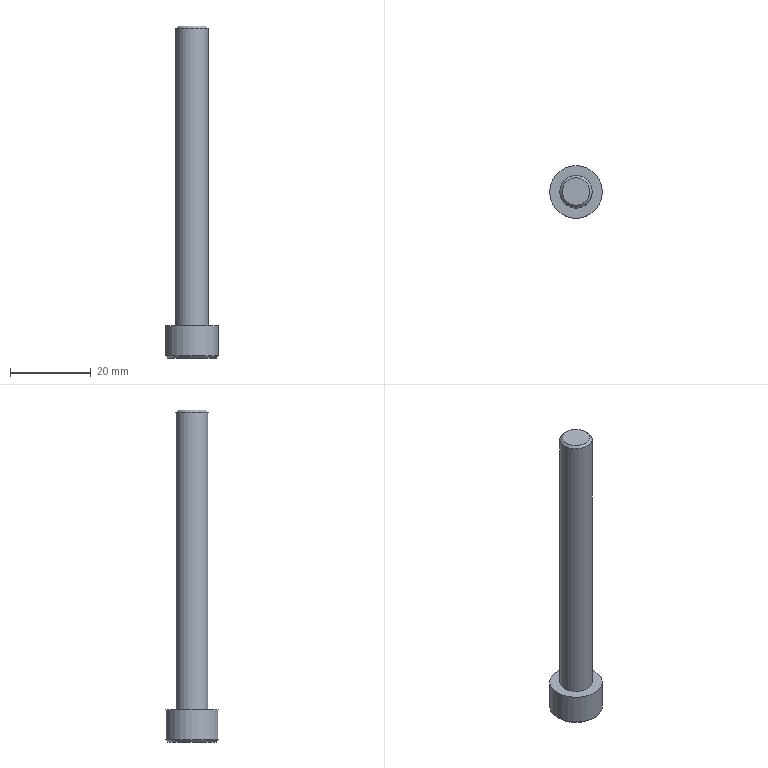Part | STEP file | gslz 2016.10.28-6_id182_x_t | 1 solid | 14 faces | box 13 x 13 x 82 mm | volume 4616 mm3 | plane 10 | cylinder 2 | cone 2 | commonest cylinder face diameters 8 x1 13 x1
STEP:
#1=CARTESIAN_POINT('',(-246.,150.,62.992));
#2=VERTEX_POINT('',#1);
#3=CARTESIAN_POINT('',(-240.,150.,62.992));
#4=DIRECTION('',(0.,0.,-1.));
#5=DIRECTION('',(-1.,0.,0.));
#6=AXIS2_PLACEMENT_3D('',#3,#4,#5);
#7=CIRCLE('',#6,6.);
#8=EDGE_CURVE('',#2,#2,#7,.T.);
#9=ORIENTED_EDGE('',*,*,#8,.T.);
#10=EDGE_LOOP('',(#9));
#11=FACE_BOUND('',#10,.T.);
#12=CARTESIAN_POINT('',(-237.,151.732,62.992));
#13=VERTEX_POINT('',#12);
#14=CARTESIAN_POINT('',(-237.,148.268,62.992));
#15=VERTEX_POINT('',#14);
#16=CARTESIAN_POINT('',(-237.,151.732,62.992));
#17=DIRECTION('',(0.,-1.,0.));
#18=VECTOR('',#17,1.);
#19=LINE('',#16,#18);
#20=EDGE_CURVE('',#13,#15,#19,.T.);
#21=ORIENTED_EDGE('',*,*,#20,.F.);
#22=CARTESIAN_POINT('',(-240.,153.464,62.992));
#23=VERTEX_POINT('',#22);
#24=CARTESIAN_POINT('',(-240.,153.464,62.992));
#25=DIRECTION('',(0.866,-0.5,0.));
#26=VECTOR('',#25,1.);
#27=LINE('',#24,#26);
#28=EDGE_CURVE('',#23,#13,#27,.T.);
#29=ORIENTED_EDGE('',*,*,#28,.F.);
#30=CARTESIAN_POINT('',(-243.,151.732,62.992));
#31=VERTEX_POINT('',#30);
#32=CARTESIAN_POINT('',(-243.,151.732,62.992));
#33=DIRECTION('',(0.866,0.5,0.));
#34=VECTOR('',#33,1.);
#35=LINE('',#32,#34);
#36=EDGE_CURVE('',#31,#23,#35,.T.);
#37=ORIENTED_EDGE('',*,*,#36,.F.);
#38=CARTESIAN_POINT('',(-243.,148.268,62.992));
#39=VERTEX_POINT('',#38);
#40=CARTESIAN_POINT('',(-243.,148.268,62.992));
#41=DIRECTION('',(0.,1.,0.));
#42=VECTOR('',#41,1.);
#43=LINE('',#40,#42);
#44=EDGE_CURVE('',#39,#31,#43,.T.);
#45=ORIENTED_EDGE('',*,*,#44,.F.);
#46=CARTESIAN_POINT('',(-240.,146.536,62.992));
#47=VERTEX_POINT('',#46);
#48=CARTESIAN_POINT('',(-240.,146.536,62.992));
#49=DIRECTION('',(-0.866,0.5,0.));
#50=VECTOR('',#49,1.);
#51=LINE('',#48,#50);
#52=EDGE_CURVE('',#47,#39,#51,.T.);
#53=ORIENTED_EDGE('',*,*,#52,.F.);
#54=CARTESIAN_POINT('',(-237.,148.268,62.992));
#55=DIRECTION('',(-0.866,-0.5,0.));
#56=VECTOR('',#55,1.);
#57=LINE('',#54,#56);
#58=EDGE_CURVE('',#15,#47,#57,.T.);
#59=ORIENTED_EDGE('',*,*,#58,.F.);
#60=EDGE_LOOP('',(#21,#29,#37,#45,#53,#59));
#61=FACE_BOUND('',#60,.T.);
#62=CARTESIAN_POINT('',(-240.,150.,62.992));
#63=DIRECTION('',(0.,0.,-1.));
#64=DIRECTION('',(1.,0.,0.));
#65=AXIS2_PLACEMENT_3D('',#62,#63,#64);
#66=PLANE('',#65);
#67=ADVANCED_FACE('',(#11,#61),#66,.T.);
#68=CARTESIAN_POINT('',(-236.6,150.,144.992));
#69=VERTEX_POINT('',#68);
#70=CARTESIAN_POINT('',(-240.,150.,144.992));
#71=DIRECTION('',(0.,0.,1.));
#72=DIRECTION('',(1.,0.,0.));
#73=AXIS2_PLACEMENT_3D('',#70,#71,#72);
#74=CIRCLE('',#73,3.4);
#75=EDGE_CURVE('',#69,#69,#74,.T.);
#76=ORIENTED_EDGE('',*,*,#75,.T.);
#77=EDGE_LOOP('',(#76));
#78=FACE_OUTER_BOUND('',#77,.T.);
#79=CARTESIAN_POINT('',(-240.,150.,144.992));
#80=DIRECTION('',(0.,0.,1.));
#81=DIRECTION('',(-1.,0.,0.));
#82=AXIS2_PLACEMENT_3D('',#79,#80,#81);
#83=PLANE('',#82);
#84=ADVANCED_FACE('',(#78),#83,.T.);
#85=CARTESIAN_POINT('',(-236.,150.,144.392));
#86=VERTEX_POINT('',#85);
#87=CARTESIAN_POINT('',(-240.,150.,144.392));
#88=DIRECTION('',(0.,0.,-1.));
#89=DIRECTION('',(1.,0.,0.));
#90=AXIS2_PLACEMENT_3D('',#87,#88,#89);
#91=CIRCLE('',#90,4.);
#92=EDGE_CURVE('',#86,#86,#91,.T.);
#93=ORIENTED_EDGE('',*,*,#92,.T.);
#94=EDGE_LOOP('',(#93));
#95=FACE_BOUND('',#94,.T.);
#96=CARTESIAN_POINT('',(-236.,150.,70.992));
#97=VERTEX_POINT('',#96);
#98=CARTESIAN_POINT('',(-240.,150.,70.992));
#99=DIRECTION('',(0.,0.,1.));
#100=DIRECTION('',(1.,0.,0.));
#101=AXIS2_PLACEMENT_3D('',#98,#99,#100);
#102=CIRCLE('',#101,4.);
#103=EDGE_CURVE('',#97,#97,#102,.T.);
#104=ORIENTED_EDGE('',*,*,#103,.T.);
#105=EDGE_LOOP('',(#104));
#106=FACE_BOUND('',#105,.T.);
#107=CARTESIAN_POINT('',(-240.,150.,129.992));
#108=DIRECTION('',(0.,0.,1.));
#109=DIRECTION('',(1.,0.,0.));
#110=AXIS2_PLACEMENT_3D('',#107,#108,#109);
#111=CYLINDRICAL_SURFACE('',#110,4.);
#112=ADVANCED_FACE('',(#95,#106),#111,.T.);
#113=ORIENTED_EDGE('',*,*,#103,.F.);
#114=EDGE_LOOP('',(#113));
#115=FACE_BOUND('',#114,.T.);
#116=CARTESIAN_POINT('',(-233.5,150.,70.992));
#117=VERTEX_POINT('',#116);
#118=CARTESIAN_POINT('',(-240.,150.,70.992));
#119=DIRECTION('',(0.,0.,1.));
#120=DIRECTION('',(1.,0.,0.));
#121=AXIS2_PLACEMENT_3D('',#118,#119,#120);
#122=CIRCLE('',#121,6.5);
#123=EDGE_CURVE('',#117,#117,#122,.T.);
#124=ORIENTED_EDGE('',*,*,#123,.T.);
#125=EDGE_LOOP('',(#124));
#126=FACE_BOUND('',#125,.T.);
#127=CARTESIAN_POINT('',(-240.,150.,70.992));
#128=DIRECTION('',(0.,0.,1.));
#129=DIRECTION('',(-1.,0.,0.));
#130=AXIS2_PLACEMENT_3D('',#127,#128,#129);
#131=PLANE('',#130);
#132=ADVANCED_FACE('',(#115,#126),#131,.T.);
#133=CARTESIAN_POINT('',(-246.5,150.,63.492));
#134=VERTEX_POINT('',#133);
#135=CARTESIAN_POINT('',(-240.,150.,63.492));
#136=DIRECTION('',(0.,0.,1.));
#137=DIRECTION('',(-1.,0.,0.));
#138=AXIS2_PLACEMENT_3D('',#135,#136,#137);
#139=CIRCLE('',#138,6.5);
#140=EDGE_CURVE('',#134,#134,#139,.T.);
#141=ORIENTED_EDGE('',*,*,#140,.T.);
#142=EDGE_LOOP('',(#141));
#143=FACE_BOUND('',#142,.T.);
#144=ORIENTED_EDGE('',*,*,#123,.F.);
#145=EDGE_LOOP('',(#144));
#146=FACE_BOUND('',#145,.T.);
#147=CARTESIAN_POINT('',(-240.,150.,59.992));
#148=DIRECTION('',(0.,0.,1.));
#149=DIRECTION('',(1.,0.,0.));
#150=AXIS2_PLACEMENT_3D('',#147,#148,#149);
#151=CYLINDRICAL_SURFACE('',#150,6.5);
#152=ADVANCED_FACE('',(#143,#146),#151,.T.);
#153=ORIENTED_EDGE('',*,*,#92,.F.);
#154=EDGE_LOOP('',(#153));
#155=FACE_BOUND('',#154,.T.);
#156=ORIENTED_EDGE('',*,*,#75,.F.);
#157=EDGE_LOOP('',(#156));
#158=FACE_BOUND('',#157,.T.);
#159=CARTESIAN_POINT('',(-240.,150.,144.992));
#160=DIRECTION('',(0.,0.,-1.));
#161=DIRECTION('',(-1.,0.,0.));
#162=AXIS2_PLACEMENT_3D('',#159,#160,#161);
#163=CONICAL_SURFACE('',#162,3.4,45.);
#164=ADVANCED_FACE('',(#155,#158),#163,.T.);
#165=ORIENTED_EDGE('',*,*,#20,.T.);
#166=CARTESIAN_POINT('',(-237.,148.268,67.992));
#167=VERTEX_POINT('',#166);
#168=CARTESIAN_POINT('',(-237.,148.268,67.992));
#169=DIRECTION('',(0.,0.,1.));
#170=VECTOR('',#169,1.);
#171=LINE('',#168,#170);
#172=EDGE_CURVE('',#15,#167,#171,.T.);
#173=ORIENTED_EDGE('',*,*,#172,.T.);
#174=CARTESIAN_POINT('',(-237.,151.732,67.992));
#175=VERTEX_POINT('',#174);
#176=CARTESIAN_POINT('',(-237.,151.732,67.992));
#177=DIRECTION('',(0.,1.,0.));
#178=VECTOR('',#177,1.);
#179=LINE('',#176,#178);
#180=EDGE_CURVE('',#167,#175,#179,.T.);
#181=ORIENTED_EDGE('',*,*,#180,.T.);
#182=CARTESIAN_POINT('',(-237.,151.732,67.992));
#183=DIRECTION('',(0.,0.,1.));
#184=VECTOR('',#183,1.);
#185=LINE('',#182,#184);
#186=EDGE_CURVE('',#13,#175,#185,.T.);
#187=ORIENTED_EDGE('',*,*,#186,.F.);
#188=EDGE_LOOP('',(#165,#173,#181,#187));
#189=FACE_OUTER_BOUND('',#188,.T.);
#190=CARTESIAN_POINT('',(-237.,151.732,67.992));
#191=DIRECTION('',(1.,0.,0.));
#192=DIRECTION('',(0.,0.,-1.));
#193=AXIS2_PLACEMENT_3D('',#190,#191,#192);
#194=PLANE('',#193);
#195=ADVANCED_FACE('',(#189),#194,.F.);
#196=ORIENTED_EDGE('',*,*,#58,.T.);
#197=CARTESIAN_POINT('',(-240.,146.536,67.992));
#198=VERTEX_POINT('',#197);
#199=CARTESIAN_POINT('',(-240.,146.536,67.992));
#200=DIRECTION('',(0.,0.,1.));
#201=VECTOR('',#200,1.);
#202=LINE('',#199,#201);
#203=EDGE_CURVE('',#47,#198,#202,.T.);
#204=ORIENTED_EDGE('',*,*,#203,.T.);
#205=CARTESIAN_POINT('',(-237.,148.268,67.992));
#206=DIRECTION('',(0.866,0.5,0.));
#207=VECTOR('',#206,1.);
#208=LINE('',#205,#207);
#209=EDGE_CURVE('',#198,#167,#208,.T.);
#210=ORIENTED_EDGE('',*,*,#209,.T.);
#211=ORIENTED_EDGE('',*,*,#172,.F.);
#212=EDGE_LOOP('',(#196,#204,#210,#211));
#213=FACE_OUTER_BOUND('',#212,.T.);
#214=CARTESIAN_POINT('',(-237.,148.268,67.992));
#215=DIRECTION('',(0.5,-0.866,0.));
#216=DIRECTION('',(0.866,0.5,0.));
#217=AXIS2_PLACEMENT_3D('',#214,#215,#216);
#218=PLANE('',#217);
#219=ADVANCED_FACE('',(#213),#218,.F.);
#220=ORIENTED_EDGE('',*,*,#52,.T.);
#221=CARTESIAN_POINT('',(-243.,148.268,67.992));
#222=VERTEX_POINT('',#221);
#223=CARTESIAN_POINT('',(-243.,148.268,67.992));
#224=DIRECTION('',(0.,0.,1.));
#225=VECTOR('',#224,1.);
#226=LINE('',#223,#225);
#227=EDGE_CURVE('',#39,#222,#226,.T.);
#228=ORIENTED_EDGE('',*,*,#227,.T.);
#229=CARTESIAN_POINT('',(-240.,146.536,67.992));
#230=DIRECTION('',(0.866,-0.5,0.));
#231=VECTOR('',#230,1.);
#232=LINE('',#229,#231);
#233=EDGE_CURVE('',#222,#198,#232,.T.);
#234=ORIENTED_EDGE('',*,*,#233,.T.);
#235=ORIENTED_EDGE('',*,*,#203,.F.);
#236=EDGE_LOOP('',(#220,#228,#234,#235));
#237=FACE_OUTER_BOUND('',#236,.T.);
#238=CARTESIAN_POINT('',(-240.,146.536,67.992));
#239=DIRECTION('',(-0.5,-0.866,0.));
#240=DIRECTION('',(0.866,-0.5,0.));
#241=AXIS2_PLACEMENT_3D('',#238,#239,#240);
#242=PLANE('',#241);
#243=ADVANCED_FACE('',(#237),#242,.F.);
#244=ORIENTED_EDGE('',*,*,#44,.T.);
#245=CARTESIAN_POINT('',(-243.,151.732,67.992));
#246=VERTEX_POINT('',#245);
#247=CARTESIAN_POINT('',(-243.,151.732,67.992));
#248=DIRECTION('',(0.,0.,1.));
#249=VECTOR('',#248,1.);
#250=LINE('',#247,#249);
#251=EDGE_CURVE('',#31,#246,#250,.T.);
#252=ORIENTED_EDGE('',*,*,#251,.T.);
#253=CARTESIAN_POINT('',(-243.,148.268,67.992));
#254=DIRECTION('',(0.,-1.,0.));
#255=VECTOR('',#254,1.);
#256=LINE('',#253,#255);
#257=EDGE_CURVE('',#246,#222,#256,.T.);
#258=ORIENTED_EDGE('',*,*,#257,.T.);
#259=ORIENTED_EDGE('',*,*,#227,.F.);
#260=EDGE_LOOP('',(#244,#252,#258,#259));
#261=FACE_OUTER_BOUND('',#260,.T.);
#262=CARTESIAN_POINT('',(-243.,148.268,67.992));
#263=DIRECTION('',(-1.,0.,0.));
#264=DIRECTION('',(0.,0.,-1.));
#265=AXIS2_PLACEMENT_3D('',#262,#263,#264);
#266=PLANE('',#265);
#267=ADVANCED_FACE('',(#261),#266,.F.);
#268=ORIENTED_EDGE('',*,*,#36,.T.);
#269=CARTESIAN_POINT('',(-240.,153.464,67.992));
#270=VERTEX_POINT('',#269);
#271=CARTESIAN_POINT('',(-240.,153.464,67.992));
#272=DIRECTION('',(0.,0.,1.));
#273=VECTOR('',#272,1.);
#274=LINE('',#271,#273);
#275=EDGE_CURVE('',#23,#270,#274,.T.);
#276=ORIENTED_EDGE('',*,*,#275,.T.);
#277=CARTESIAN_POINT('',(-243.,151.732,67.992));
#278=DIRECTION('',(-0.866,-0.5,0.));
#279=VECTOR('',#278,1.);
#280=LINE('',#277,#279);
#281=EDGE_CURVE('',#270,#246,#280,.T.);
#282=ORIENTED_EDGE('',*,*,#281,.T.);
#283=ORIENTED_EDGE('',*,*,#251,.F.);
#284=EDGE_LOOP('',(#268,#276,#282,#283));
#285=FACE_OUTER_BOUND('',#284,.T.);
#286=CARTESIAN_POINT('',(-243.,151.732,67.992));
#287=DIRECTION('',(-0.5,0.866,0.));
#288=DIRECTION('',(-0.866,-0.5,0.));
#289=AXIS2_PLACEMENT_3D('',#286,#287,#288);
#290=PLANE('',#289);
#291=ADVANCED_FACE('',(#285),#290,.F.);
#292=ORIENTED_EDGE('',*,*,#28,.T.);
#293=ORIENTED_EDGE('',*,*,#186,.T.);
#294=CARTESIAN_POINT('',(-240.,153.464,67.992));
#295=DIRECTION('',(-0.866,0.5,0.));
#296=VECTOR('',#295,1.);
#297=LINE('',#294,#296);
#298=EDGE_CURVE('',#175,#270,#297,.T.);
#299=ORIENTED_EDGE('',*,*,#298,.T.);
#300=ORIENTED_EDGE('',*,*,#275,.F.);
#301=EDGE_LOOP('',(#292,#293,#299,#300));
#302=FACE_OUTER_BOUND('',#301,.T.);
#303=CARTESIAN_POINT('',(-240.,153.464,67.992));
#304=DIRECTION('',(0.5,0.866,0.));
#305=DIRECTION('',(-0.866,0.5,0.));
#306=AXIS2_PLACEMENT_3D('',#303,#304,#305);
#307=PLANE('',#306);
#308=ADVANCED_FACE('',(#302),#307,.F.);
#309=ORIENTED_EDGE('',*,*,#180,.F.);
#310=ORIENTED_EDGE('',*,*,#209,.F.);
#311=ORIENTED_EDGE('',*,*,#233,.F.);
#312=ORIENTED_EDGE('',*,*,#257,.F.);
#313=ORIENTED_EDGE('',*,*,#281,.F.);
#314=ORIENTED_EDGE('',*,*,#298,.F.);
#315=EDGE_LOOP('',(#309,#310,#311,#312,#313,#314));
#316=FACE_OUTER_BOUND('',#315,.T.);
#317=CARTESIAN_POINT('',(-237.,148.268,67.992));
#318=DIRECTION('',(0.,0.,-1.));
#319=DIRECTION('',(1.,0.,0.));
#320=AXIS2_PLACEMENT_3D('',#317,#318,#319);
#321=PLANE('',#320);
#322=ADVANCED_FACE('',(#316),#321,.T.);
#323=ORIENTED_EDGE('',*,*,#8,.F.);
#324=EDGE_LOOP('',(#323));
#325=FACE_BOUND('',#324,.T.);
#326=ORIENTED_EDGE('',*,*,#140,.F.);
#327=EDGE_LOOP('',(#326));
#328=FACE_BOUND('',#327,.T.);
#329=CARTESIAN_POINT('',(-240.,150.,63.492));
#330=DIRECTION('',(0.,0.,1.));
#331=DIRECTION('',(1.,0.,0.));
#332=AXIS2_PLACEMENT_3D('',#329,#330,#331);
#333=CONICAL_SURFACE('',#332,6.5,45.);
#334=ADVANCED_FACE('',(#325,#328),#333,.T.);
#335=CLOSED_SHELL('',(#67,#84,#112,#132,#152,#164,#195,#219,#243,#267,#291,#308,#322,#334));
#336=MANIFOLD_SOLID_BREP('',#335);
#337=(LENGTH_UNIT()NAMED_UNIT(*)SI_UNIT(.MILLI.,.METRE.));
#338=UNCERTAINTY_MEASURE_WITH_UNIT(LENGTH_MEASURE(0.00002),#337,'','');
#339=(NAMED_UNIT(*)PLANE_ANGLE_UNIT()SI_UNIT($,.RADIAN.));
#340=PLANE_ANGLE_MEASURE_WITH_UNIT(PLANE_ANGLE_MEASURE(0.01745),#339);
#341=DIMENSIONAL_EXPONENTS(0.,0.,0.,0.,0.,0.,0.);
#342=(CONVERSION_BASED_UNIT('DEGREE',#340)NAMED_UNIT(#341)PLANE_ANGLE_UNIT());
#343=(NAMED_UNIT(*)SI_UNIT($,.STERADIAN.)SOLID_ANGLE_UNIT());
#344=(GEOMETRIC_REPRESENTATION_CONTEXT(3)GLOBAL_UNCERTAINTY_ASSIGNED_CONTEXT((#338))GLOBAL_UNIT_ASSIGNED_CONTEXT((#337,#342,#343))REPRESENTATION_CONTEXT('',''));
#345=ADVANCED_BREP_SHAPE_REPRESENTATION('',(#336),#344);